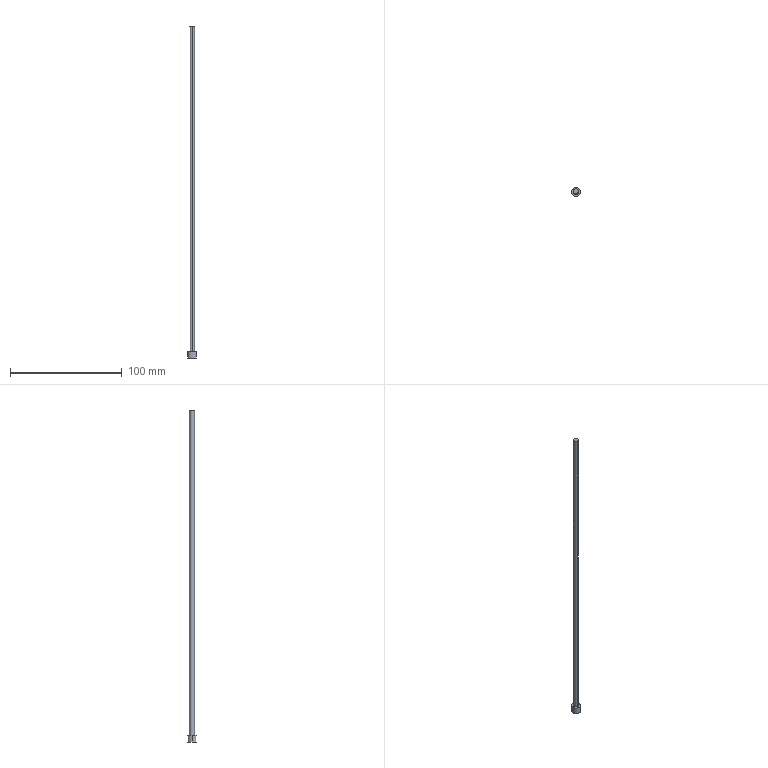Part | Creo | 1 solid | 7 faces | box 8 x 8 x 297.407 mm | volume 4936 mm3 | cylinder 4 | plane 3 | commonest cylinder face diameters 4.5 x2 8 x2
STEP:
#1=CARTESIAN_POINT('',(50.55,-133.,1.407));
#2=VERTEX_POINT('',#1);
#3=CARTESIAN_POINT('',(48.3,-130.75,1.407));
#4=VERTEX_POINT('',#3);
#5=CARTESIAN_POINT('',(48.3,-133.,1.407));
#6=DIRECTION('',(0.,0.,1.));
#7=DIRECTION('',(1.,0.,0.));
#8=AXIS2_PLACEMENT_3D('',#5,#6,#7);
#9=CIRCLE('',#8,2.25);
#10=EDGE_CURVE('',#2,#4,#9,.T.);
#11=ORIENTED_EDGE('',*,*,#10,.F.);
#12=CARTESIAN_POINT('',(48.3,-135.25,1.407));
#13=VERTEX_POINT('',#12);
#14=CARTESIAN_POINT('',(48.3,-133.,1.407));
#15=DIRECTION('',(0.,0.,1.));
#16=DIRECTION('',(0.,-1.,0.));
#17=AXIS2_PLACEMENT_3D('',#14,#15,#16);
#18=CIRCLE('',#17,2.25);
#19=EDGE_CURVE('',#13,#2,#18,.T.);
#20=ORIENTED_EDGE('',*,*,#19,.F.);
#21=CARTESIAN_POINT('',(48.3,-133.,1.407));
#22=DIRECTION('',(0.,0.,1.));
#23=DIRECTION('',(0.,1.,0.));
#24=AXIS2_PLACEMENT_3D('',#21,#22,#23);
#25=CIRCLE('',#24,2.25);
#26=EDGE_CURVE('',#4,#13,#25,.T.);
#27=ORIENTED_EDGE('',*,*,#26,.F.);
#28=EDGE_LOOP('',(#11,#20,#27));
#29=FACE_OUTER_BOUND('',#28,.F.);
#30=CARTESIAN_POINT('',(60.804,-218.798,1.407));
#31=DIRECTION('',(0.,0.,1.));
#32=DIRECTION('',(-1.,0.,0.));
#33=AXIS2_PLACEMENT_3D('',#30,#31,#32);
#34=PLANE('',#33);
#35=ADVANCED_FACE('',(#29),#34,.T.);
#36=CARTESIAN_POINT('',(48.3,-130.75,-290.));
#37=VERTEX_POINT('',#36);
#38=CARTESIAN_POINT('',(50.55,-133.,-290.));
#39=VERTEX_POINT('',#38);
#40=CARTESIAN_POINT('',(48.3,-133.,-290.));
#41=DIRECTION('',(0.,0.,-1.));
#42=DIRECTION('',(0.,1.,0.));
#43=AXIS2_PLACEMENT_3D('',#40,#41,#42);
#44=CIRCLE('',#43,2.25);
#45=EDGE_CURVE('',#37,#39,#44,.T.);
#46=ORIENTED_EDGE('',*,*,#45,.T.);
#47=CARTESIAN_POINT('',(48.3,-135.25,-290.));
#48=VERTEX_POINT('',#47);
#49=CARTESIAN_POINT('',(48.3,-133.,-290.));
#50=DIRECTION('',(0.,0.,-1.));
#51=DIRECTION('',(1.,0.,0.));
#52=AXIS2_PLACEMENT_3D('',#49,#50,#51);
#53=CIRCLE('',#52,2.25);
#54=EDGE_CURVE('',#39,#48,#53,.T.);
#55=ORIENTED_EDGE('',*,*,#54,.T.);
#56=CARTESIAN_POINT('',(48.3,-135.25,-290.));
#57=DIRECTION('',(0.,0.,1.));
#58=VECTOR('',#57,291.407);
#59=LINE('',#56,#58);
#60=EDGE_CURVE('',#48,#13,#59,.T.);
#61=ORIENTED_EDGE('',*,*,#60,.T.);
#62=ORIENTED_EDGE('',*,*,#19,.T.);
#63=ORIENTED_EDGE('',*,*,#10,.T.);
#64=CARTESIAN_POINT('',(48.3,-130.75,-290.));
#65=DIRECTION('',(0.,0.,1.));
#66=VECTOR('',#65,291.407);
#67=LINE('',#64,#66);
#68=EDGE_CURVE('',#37,#4,#67,.T.);
#69=ORIENTED_EDGE('',*,*,#68,.F.);
#70=EDGE_LOOP('',(#46,#55,#61,#62,#63,#69));
#71=FACE_OUTER_BOUND('',#70,.F.);
#72=CARTESIAN_POINT('',(48.3,-133.,-337.475));
#73=DIRECTION('',(0.,0.,1.));
#74=DIRECTION('',(0.,-1.,0.));
#75=AXIS2_PLACEMENT_3D('',#72,#73,#74);
#76=CYLINDRICAL_SURFACE('',#75,2.25);
#77=ADVANCED_FACE('',(#71),#76,.T.);
#78=CARTESIAN_POINT('',(52.3,-133.,-290.));
#79=VERTEX_POINT('',#78);
#80=CARTESIAN_POINT('',(44.3,-133.,-290.));
#81=VERTEX_POINT('',#80);
#82=CARTESIAN_POINT('',(48.3,-133.,-290.));
#83=DIRECTION('',(0.,0.,1.));
#84=DIRECTION('',(1.,0.,0.));
#85=AXIS2_PLACEMENT_3D('',#82,#83,#84);
#86=CIRCLE('',#85,4.);
#87=EDGE_CURVE('',#79,#81,#86,.T.);
#88=ORIENTED_EDGE('',*,*,#87,.F.);
#89=CARTESIAN_POINT('',(48.3,-133.,-290.));
#90=DIRECTION('',(0.,0.,1.));
#91=DIRECTION('',(-1.,0.,0.));
#92=AXIS2_PLACEMENT_3D('',#89,#90,#91);
#93=CIRCLE('',#92,4.);
#94=EDGE_CURVE('',#81,#79,#93,.T.);
#95=ORIENTED_EDGE('',*,*,#94,.F.);
#96=EDGE_LOOP('',(#88,#95));
#97=FACE_OUTER_BOUND('',#96,.F.);
#98=ORIENTED_EDGE('',*,*,#54,.F.);
#99=ORIENTED_EDGE('',*,*,#45,.F.);
#100=CARTESIAN_POINT('',(48.3,-133.,-290.));
#101=DIRECTION('',(0.,0.,-1.));
#102=DIRECTION('',(0.,-1.,0.));
#103=AXIS2_PLACEMENT_3D('',#100,#101,#102);
#104=CIRCLE('',#103,2.25);
#105=EDGE_CURVE('',#48,#37,#104,.T.);
#106=ORIENTED_EDGE('',*,*,#105,.F.);
#107=EDGE_LOOP('',(#98,#99,#106));
#108=FACE_BOUND('',#107,.F.);
#109=CARTESIAN_POINT('',(48.3,-133.,-290.));
#110=DIRECTION('',(0.,0.,1.));
#111=DIRECTION('',(-1.,0.,0.));
#112=AXIS2_PLACEMENT_3D('',#109,#110,#111);
#113=PLANE('',#112);
#114=ADVANCED_FACE('',(#97,#108),#113,.T.);
#115=ORIENTED_EDGE('',*,*,#105,.T.);
#116=ORIENTED_EDGE('',*,*,#68,.T.);
#117=ORIENTED_EDGE('',*,*,#26,.T.);
#118=ORIENTED_EDGE('',*,*,#60,.F.);
#119=EDGE_LOOP('',(#115,#116,#117,#118));
#120=FACE_OUTER_BOUND('',#119,.F.);
#121=CARTESIAN_POINT('',(48.3,-133.,-337.475));
#122=DIRECTION('',(0.,0.,1.));
#123=DIRECTION('',(0.,-1.,0.));
#124=AXIS2_PLACEMENT_3D('',#121,#122,#123);
#125=CYLINDRICAL_SURFACE('',#124,2.25);
#126=ADVANCED_FACE('',(#120),#125,.T.);
#127=ORIENTED_EDGE('',*,*,#87,.T.);
#128=CARTESIAN_POINT('',(44.3,-133.,-296.));
#129=VERTEX_POINT('',#128);
#130=CARTESIAN_POINT('',(44.3,-133.,-296.));
#131=DIRECTION('',(0.,0.,1.));
#132=VECTOR('',#131,6.);
#133=LINE('',#130,#132);
#134=EDGE_CURVE('',#129,#81,#133,.T.);
#135=ORIENTED_EDGE('',*,*,#134,.F.);
#136=CARTESIAN_POINT('',(52.3,-133.,-296.));
#137=VERTEX_POINT('',#136);
#138=CARTESIAN_POINT('',(48.3,-133.,-296.));
#139=DIRECTION('',(0.,0.,-1.));
#140=DIRECTION('',(-1.,0.,0.));
#141=AXIS2_PLACEMENT_3D('',#138,#139,#140);
#142=CIRCLE('',#141,4.);
#143=EDGE_CURVE('',#129,#137,#142,.T.);
#144=ORIENTED_EDGE('',*,*,#143,.T.);
#145=CARTESIAN_POINT('',(52.3,-133.,-296.));
#146=DIRECTION('',(0.,0.,1.));
#147=VECTOR('',#146,6.);
#148=LINE('',#145,#147);
#149=EDGE_CURVE('',#137,#79,#148,.T.);
#150=ORIENTED_EDGE('',*,*,#149,.T.);
#151=EDGE_LOOP('',(#127,#135,#144,#150));
#152=FACE_OUTER_BOUND('',#151,.F.);
#153=CARTESIAN_POINT('',(48.3,-133.,-296.));
#154=DIRECTION('',(0.,0.,1.));
#155=DIRECTION('',(-1.,0.,0.));
#156=AXIS2_PLACEMENT_3D('',#153,#154,#155);
#157=CYLINDRICAL_SURFACE('',#156,4.);
#158=ADVANCED_FACE('',(#152),#157,.T.);
#159=ORIENTED_EDGE('',*,*,#94,.T.);
#160=ORIENTED_EDGE('',*,*,#149,.F.);
#161=CARTESIAN_POINT('',(48.3,-133.,-296.));
#162=DIRECTION('',(0.,0.,-1.));
#163=DIRECTION('',(1.,0.,0.));
#164=AXIS2_PLACEMENT_3D('',#161,#162,#163);
#165=CIRCLE('',#164,4.);
#166=EDGE_CURVE('',#137,#129,#165,.T.);
#167=ORIENTED_EDGE('',*,*,#166,.T.);
#168=ORIENTED_EDGE('',*,*,#134,.T.);
#169=EDGE_LOOP('',(#159,#160,#167,#168));
#170=FACE_OUTER_BOUND('',#169,.F.);
#171=CARTESIAN_POINT('',(48.3,-133.,-296.));
#172=DIRECTION('',(0.,0.,1.));
#173=DIRECTION('',(-1.,0.,0.));
#174=AXIS2_PLACEMENT_3D('',#171,#172,#173);
#175=CYLINDRICAL_SURFACE('',#174,4.);
#176=ADVANCED_FACE('',(#170),#175,.T.);
#177=ORIENTED_EDGE('',*,*,#166,.F.);
#178=ORIENTED_EDGE('',*,*,#143,.F.);
#179=EDGE_LOOP('',(#177,#178));
#180=FACE_OUTER_BOUND('',#179,.F.);
#181=CARTESIAN_POINT('',(10.,0.004699,-296.));
#182=DIRECTION('',(0.,0.,1.));
#183=DIRECTION('',(0.,-1.,0.));
#184=AXIS2_PLACEMENT_3D('',#181,#182,#183);
#185=PLANE('',#184);
#186=ADVANCED_FACE('',(#180),#185,.F.);
#187=CLOSED_SHELL('',(#35,#77,#114,#126,#158,#176,#186));
#188=MANIFOLD_SOLID_BREP('',#187);
#189=(LENGTH_UNIT()NAMED_UNIT(*)SI_UNIT(.MILLI.,.METRE.));
#190=UNCERTAINTY_MEASURE_WITH_UNIT(LENGTH_MEASURE(0.02976),#189,'','');
#191=(NAMED_UNIT(*)PLANE_ANGLE_UNIT()SI_UNIT($,.RADIAN.));
#192=PLANE_ANGLE_MEASURE_WITH_UNIT(PLANE_ANGLE_MEASURE(0.01745),#191);
#193=(CONVERSION_BASED_UNIT('DEGREE',#192)NAMED_UNIT(*)PLANE_ANGLE_UNIT());
#194=(NAMED_UNIT(*)SI_UNIT($,.STERADIAN.)SOLID_ANGLE_UNIT());
#195=(GEOMETRIC_REPRESENTATION_CONTEXT(3)GLOBAL_UNCERTAINTY_ASSIGNED_CONTEXT((#190))GLOBAL_UNIT_ASSIGNED_CONTEXT((#189,#193,#194))REPRESENTATION_CONTEXT('',''));
#196=ADVANCED_BREP_SHAPE_REPRESENTATION('',(#188),#195);